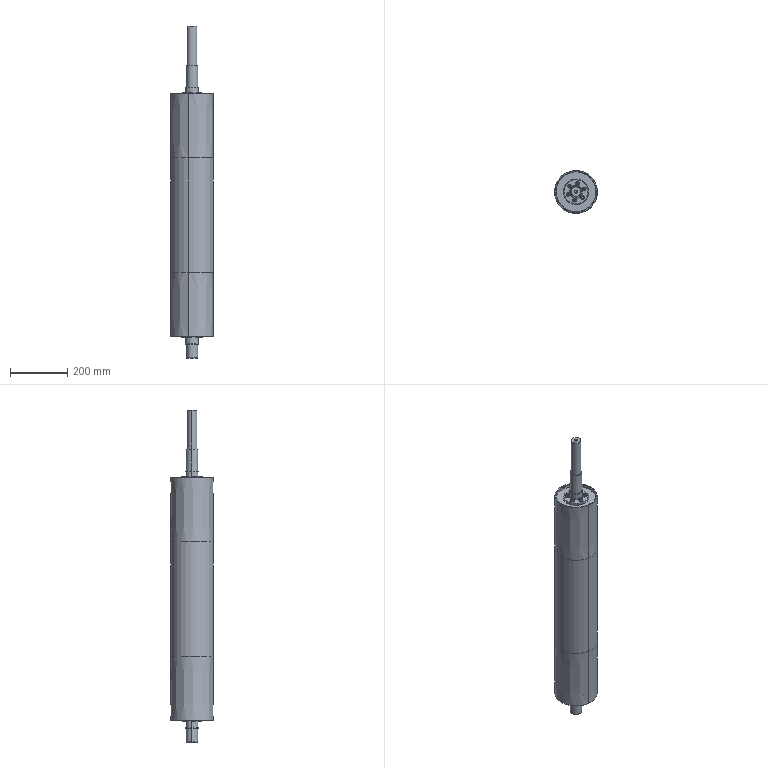Part | SolidWorks | 20 solids | 401 faces | box 150 x 150 x 1164 mm | volume 4781724 mm3 | plane 146 | cylinder 143 | cone 62 | torus 50 | commonest cylinder face diameters 6.647 x44 8 x24 13 x24 75 x8 140 x8 45 x6